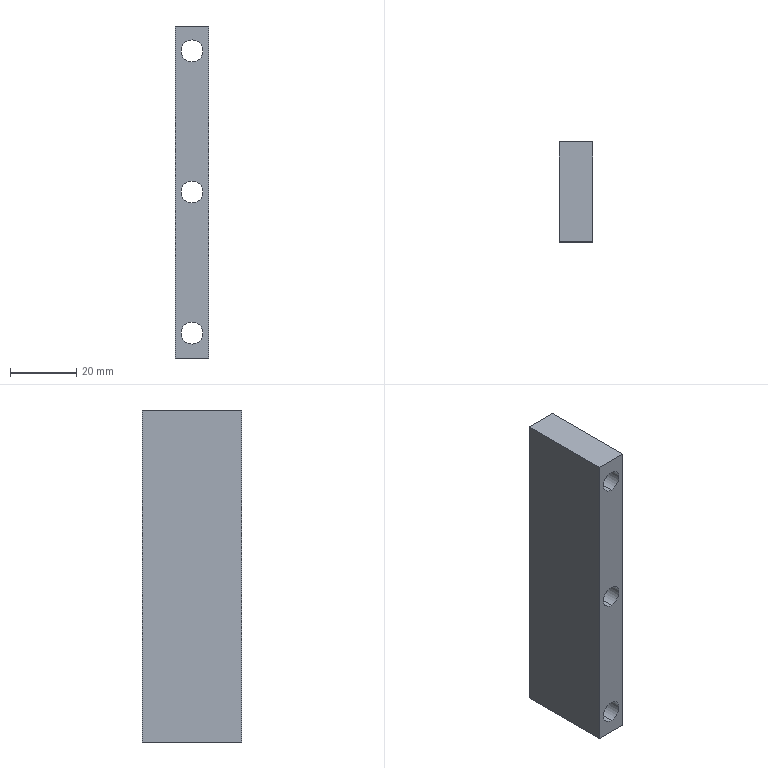Part | STEP file | 0-09-15 Support plate | 1 solid | 12 faces | box 10 x 30 x 100 mm | volume 26921 mm3 | cylinder 6 | plane 6 | commonest cylinder face diameters 6.6 x6
STEP:
#1=CARTESIAN_POINT('',(0.,0.,0.));
#2=DIRECTION('',(0.,0.,1.));
#3=DIRECTION('',(1.,0.,0.));
#4=AXIS2_PLACEMENT_3D('',#1,#2,#3);
#5=CARTESIAN_POINT('',(0.,-15.,-39.2));
#6=VERTEX_POINT('',#5);
#7=CARTESIAN_POINT('',(0.,15.,-39.2));
#8=VERTEX_POINT('',#7);
#9=CARTESIAN_POINT('',(0.,15.,-39.2));
#10=DIRECTION('',(0.,1.,0.));
#11=VECTOR('',#10,1.);
#12=LINE('',#9,#11);
#13=CARTESIAN_POINT('',(0.,15.,-42.5));
#14=DIRECTION('',(0.,1.,0.));
#15=DIRECTION('',(0.,0.,1.));
#16=AXIS2_PLACEMENT_3D('',#13,#14,#15);
#17=CYLINDRICAL_SURFACE('',#16,3.3);
#18=CARTESIAN_POINT('',(6.283,0.));
#19=DIRECTION('',(0.,1.));
#20=VECTOR('',#19,1.);
#21=LINE('',#18,#20);
#22=(GEOMETRIC_REPRESENTATION_CONTEXT(2)PARAMETRIC_REPRESENTATION_CONTEXT()REPRESENTATION_CONTEXT('',''));
#23=DEFINITIONAL_REPRESENTATION('',(#21),#22);
#24=PCURVE('',#17,#23);
#25=CARTESIAN_POINT('',(0.,15.,-42.5));
#26=DIRECTION('',(0.,1.,0.));
#27=DIRECTION('',(0.,0.,1.));
#28=AXIS2_PLACEMENT_3D('',#25,#26,#27);
#29=CYLINDRICAL_SURFACE('',#28,3.3);
#30=CARTESIAN_POINT('',(0.,0.));
#31=DIRECTION('',(0.,1.));
#32=VECTOR('',#31,1.);
#33=LINE('',#30,#32);
#34=(GEOMETRIC_REPRESENTATION_CONTEXT(2)PARAMETRIC_REPRESENTATION_CONTEXT()REPRESENTATION_CONTEXT('',''));
#35=DEFINITIONAL_REPRESENTATION('',(#33),#34);
#36=PCURVE('',#29,#35);
#37=SURFACE_CURVE('',#12,(#24,#36),.PCURVE_S1.);
#38=EDGE_CURVE('',#6,#8,#37,.T.);
#39=ORIENTED_EDGE('',*,*,#38,.T.);
#40=CARTESIAN_POINT('',(0.,15.,-45.8));
#41=VERTEX_POINT('',#40);
#42=CARTESIAN_POINT('',(0.,15.,-42.5));
#43=DIRECTION('',(0.,1.,0.));
#44=DIRECTION('',(0.,0.,1.));
#45=AXIS2_PLACEMENT_3D('',#42,#43,#44);
#46=CIRCLE('',#45,3.3);
#47=CARTESIAN_POINT('',(0.,0.));
#48=DIRECTION('',(1.,0.));
#49=VECTOR('',#48,1.);
#50=LINE('',#47,#49);
#51=(GEOMETRIC_REPRESENTATION_CONTEXT(2)PARAMETRIC_REPRESENTATION_CONTEXT()REPRESENTATION_CONTEXT('',''));
#52=DEFINITIONAL_REPRESENTATION('',(#50),#51);
#53=PCURVE('',#17,#52);
#54=CARTESIAN_POINT('',(5.,15.,-50.));
#55=DIRECTION('',(0.,-1.,0.));
#56=DIRECTION('',(0.,0.,-1.));
#57=AXIS2_PLACEMENT_3D('',#54,#55,#56);
#58=PLANE('',#57);
#59=CARTESIAN_POINT('',(-10.8,-5.));
#60=CARTESIAN_POINT('',(-10.8,0.7158));
#61=CARTESIAN_POINT('',(-5.85,-2.142));
#62=CARTESIAN_POINT('',(-0.9,-5.));
#63=CARTESIAN_POINT('',(-5.85,-7.858));
#64=CARTESIAN_POINT('',(-10.8,-10.716));
#65=CARTESIAN_POINT('',(-10.8,-5.));
#66=(BOUNDED_CURVE()B_SPLINE_CURVE(2,(#59,#60,#61,#62,#63,#64,#65),.UNSPECIFIED.,.T.,.F.)B_SPLINE_CURVE_WITH_KNOTS((1,2,2,2,2,1),(-2.094,0.,2.094,4.189,6.283,8.378),.UNSPECIFIED.)CURVE()GEOMETRIC_REPRESENTATION_ITEM()RATIONAL_B_SPLINE_CURVE((1.,0.5,1.,0.5,1.,0.5,1.))REPRESENTATION_ITEM(''));
#67=(GEOMETRIC_REPRESENTATION_CONTEXT(2)PARAMETRIC_REPRESENTATION_CONTEXT()REPRESENTATION_CONTEXT('',''));
#68=DEFINITIONAL_REPRESENTATION('',(#66),#67);
#69=PCURVE('',#58,#68);
#70=SURFACE_CURVE('',#46,(#53,#69),.PCURVE_S1.);
#71=EDGE_CURVE('',#41,#8,#70,.T.);
#72=ORIENTED_EDGE('',*,*,#71,.F.);
#73=CARTESIAN_POINT('',(0.,-15.,-45.8));
#74=VERTEX_POINT('',#73);
#75=CARTESIAN_POINT('',(0.,15.,-45.8));
#76=DIRECTION('',(0.,1.,0.));
#77=VECTOR('',#76,1.);
#78=LINE('',#75,#77);
#79=CARTESIAN_POINT('',(3.142,0.));
#80=DIRECTION('',(0.,1.));
#81=VECTOR('',#80,1.);
#82=LINE('',#79,#81);
#83=(GEOMETRIC_REPRESENTATION_CONTEXT(2)PARAMETRIC_REPRESENTATION_CONTEXT()REPRESENTATION_CONTEXT('',''));
#84=DEFINITIONAL_REPRESENTATION('',(#82),#83);
#85=PCURVE('',#17,#84);
#86=CARTESIAN_POINT('',(3.142,0.));
#87=DIRECTION('',(0.,1.));
#88=VECTOR('',#87,1.);
#89=LINE('',#86,#88);
#90=(GEOMETRIC_REPRESENTATION_CONTEXT(2)PARAMETRIC_REPRESENTATION_CONTEXT()REPRESENTATION_CONTEXT('',''));
#91=DEFINITIONAL_REPRESENTATION('',(#89),#90);
#92=PCURVE('',#29,#91);
#93=SURFACE_CURVE('',#78,(#85,#92),.PCURVE_S1.);
#94=EDGE_CURVE('',#74,#41,#93,.T.);
#95=ORIENTED_EDGE('',*,*,#94,.F.);
#96=CARTESIAN_POINT('',(0.,-15.,-42.5));
#97=DIRECTION('',(0.,1.,0.));
#98=DIRECTION('',(0.,0.,1.));
#99=AXIS2_PLACEMENT_3D('',#96,#97,#98);
#100=CIRCLE('',#99,3.3);
#101=CARTESIAN_POINT('',(0.,-30.));
#102=DIRECTION('',(1.,0.));
#103=VECTOR('',#102,1.);
#104=LINE('',#101,#103);
#105=(GEOMETRIC_REPRESENTATION_CONTEXT(2)PARAMETRIC_REPRESENTATION_CONTEXT()REPRESENTATION_CONTEXT('',''));
#106=DEFINITIONAL_REPRESENTATION('',(#104),#105);
#107=PCURVE('',#17,#106);
#108=CARTESIAN_POINT('',(5.,-15.,-50.));
#109=DIRECTION('',(0.,1.,0.));
#110=DIRECTION('',(0.,0.,1.));
#111=AXIS2_PLACEMENT_3D('',#108,#109,#110);
#112=PLANE('',#111);
#113=CARTESIAN_POINT('',(7.5,-5.));
#114=DIRECTION('',(1.,0.));
#115=AXIS2_PLACEMENT_2D('',#113,#114);
#116=CIRCLE('',#115,3.3);
#117=(GEOMETRIC_REPRESENTATION_CONTEXT(2)PARAMETRIC_REPRESENTATION_CONTEXT()REPRESENTATION_CONTEXT('',''));
#118=DEFINITIONAL_REPRESENTATION('',(#116),#117);
#119=PCURVE('',#112,#118);
#120=SURFACE_CURVE('',#100,(#107,#119),.PCURVE_S1.);
#121=EDGE_CURVE('',#74,#6,#120,.T.);
#122=ORIENTED_EDGE('',*,*,#121,.T.);
#123=EDGE_LOOP('',(#39,#72,#95,#122));
#124=FACE_BOUND('',#123,.F.);
#125=ADVANCED_FACE('',(#124),#17,.F.);
#126=CARTESIAN_POINT('',(0.,-15.,3.3));
#127=VERTEX_POINT('',#126);
#128=CARTESIAN_POINT('',(0.,15.,3.3));
#129=VERTEX_POINT('',#128);
#130=CARTESIAN_POINT('',(0.,15.,3.3));
#131=DIRECTION('',(0.,1.,0.));
#132=VECTOR('',#131,1.);
#133=LINE('',#130,#132);
#134=CARTESIAN_POINT('',(0.,15.,0.));
#135=DIRECTION('',(0.,1.,0.));
#136=DIRECTION('',(0.,0.,1.));
#137=AXIS2_PLACEMENT_3D('',#134,#135,#136);
#138=CYLINDRICAL_SURFACE('',#137,3.3);
#139=CARTESIAN_POINT('',(6.283,0.));
#140=DIRECTION('',(0.,1.));
#141=VECTOR('',#140,1.);
#142=LINE('',#139,#141);
#143=(GEOMETRIC_REPRESENTATION_CONTEXT(2)PARAMETRIC_REPRESENTATION_CONTEXT()REPRESENTATION_CONTEXT('',''));
#144=DEFINITIONAL_REPRESENTATION('',(#142),#143);
#145=PCURVE('',#138,#144);
#146=CARTESIAN_POINT('',(0.,15.,0.));
#147=DIRECTION('',(0.,1.,0.));
#148=DIRECTION('',(0.,0.,1.));
#149=AXIS2_PLACEMENT_3D('',#146,#147,#148);
#150=CYLINDRICAL_SURFACE('',#149,3.3);
#151=CARTESIAN_POINT('',(0.,0.));
#152=DIRECTION('',(0.,1.));
#153=VECTOR('',#152,1.);
#154=LINE('',#151,#153);
#155=(GEOMETRIC_REPRESENTATION_CONTEXT(2)PARAMETRIC_REPRESENTATION_CONTEXT()REPRESENTATION_CONTEXT('',''));
#156=DEFINITIONAL_REPRESENTATION('',(#154),#155);
#157=PCURVE('',#150,#156);
#158=SURFACE_CURVE('',#133,(#145,#157),.PCURVE_S1.);
#159=EDGE_CURVE('',#127,#129,#158,.T.);
#160=ORIENTED_EDGE('',*,*,#159,.T.);
#161=CARTESIAN_POINT('',(0.,15.,-3.3));
#162=VERTEX_POINT('',#161);
#163=CARTESIAN_POINT('',(0.,15.,0.));
#164=DIRECTION('',(0.,1.,0.));
#165=DIRECTION('',(0.,0.,1.));
#166=AXIS2_PLACEMENT_3D('',#163,#164,#165);
#167=CIRCLE('',#166,3.3);
#168=CARTESIAN_POINT('',(0.,0.));
#169=DIRECTION('',(1.,0.));
#170=VECTOR('',#169,1.);
#171=LINE('',#168,#170);
#172=(GEOMETRIC_REPRESENTATION_CONTEXT(2)PARAMETRIC_REPRESENTATION_CONTEXT()REPRESENTATION_CONTEXT('',''));
#173=DEFINITIONAL_REPRESENTATION('',(#171),#172);
#174=PCURVE('',#138,#173);
#175=CARTESIAN_POINT('',(-53.3,-5.));
#176=CARTESIAN_POINT('',(-53.3,0.7158));
#177=CARTESIAN_POINT('',(-48.35,-2.142));
#178=CARTESIAN_POINT('',(-43.4,-5.));
#179=CARTESIAN_POINT('',(-48.35,-7.858));
#180=CARTESIAN_POINT('',(-53.3,-10.716));
#181=CARTESIAN_POINT('',(-53.3,-5.));
#182=(BOUNDED_CURVE()B_SPLINE_CURVE(2,(#175,#176,#177,#178,#179,#180,#181),.UNSPECIFIED.,.T.,.F.)B_SPLINE_CURVE_WITH_KNOTS((1,2,2,2,2,1),(-2.094,0.,2.094,4.189,6.283,8.378),.UNSPECIFIED.)CURVE()GEOMETRIC_REPRESENTATION_ITEM()RATIONAL_B_SPLINE_CURVE((1.,0.5,1.,0.5,1.,0.5,1.))REPRESENTATION_ITEM(''));
#183=(GEOMETRIC_REPRESENTATION_CONTEXT(2)PARAMETRIC_REPRESENTATION_CONTEXT()REPRESENTATION_CONTEXT('',''));
#184=DEFINITIONAL_REPRESENTATION('',(#182),#183);
#185=PCURVE('',#58,#184);
#186=SURFACE_CURVE('',#167,(#174,#185),.PCURVE_S1.);
#187=EDGE_CURVE('',#162,#129,#186,.T.);
#188=ORIENTED_EDGE('',*,*,#187,.F.);
#189=CARTESIAN_POINT('',(0.,-15.,-3.3));
#190=VERTEX_POINT('',#189);
#191=CARTESIAN_POINT('',(0.,15.,-3.3));
#192=DIRECTION('',(0.,1.,0.));
#193=VECTOR('',#192,1.);
#194=LINE('',#191,#193);
#195=CARTESIAN_POINT('',(3.142,0.));
#196=DIRECTION('',(0.,1.));
#197=VECTOR('',#196,1.);
#198=LINE('',#195,#197);
#199=(GEOMETRIC_REPRESENTATION_CONTEXT(2)PARAMETRIC_REPRESENTATION_CONTEXT()REPRESENTATION_CONTEXT('',''));
#200=DEFINITIONAL_REPRESENTATION('',(#198),#199);
#201=PCURVE('',#138,#200);
#202=CARTESIAN_POINT('',(3.142,0.));
#203=DIRECTION('',(0.,1.));
#204=VECTOR('',#203,1.);
#205=LINE('',#202,#204);
#206=(GEOMETRIC_REPRESENTATION_CONTEXT(2)PARAMETRIC_REPRESENTATION_CONTEXT()REPRESENTATION_CONTEXT('',''));
#207=DEFINITIONAL_REPRESENTATION('',(#205),#206);
#208=PCURVE('',#150,#207);
#209=SURFACE_CURVE('',#194,(#201,#208),.PCURVE_S1.);
#210=EDGE_CURVE('',#190,#162,#209,.T.);
#211=ORIENTED_EDGE('',*,*,#210,.F.);
#212=CARTESIAN_POINT('',(0.,-15.,0.));
#213=DIRECTION('',(0.,1.,0.));
#214=DIRECTION('',(0.,0.,1.));
#215=AXIS2_PLACEMENT_3D('',#212,#213,#214);
#216=CIRCLE('',#215,3.3);
#217=CARTESIAN_POINT('',(0.,-30.));
#218=DIRECTION('',(1.,0.));
#219=VECTOR('',#218,1.);
#220=LINE('',#217,#219);
#221=(GEOMETRIC_REPRESENTATION_CONTEXT(2)PARAMETRIC_REPRESENTATION_CONTEXT()REPRESENTATION_CONTEXT('',''));
#222=DEFINITIONAL_REPRESENTATION('',(#220),#221);
#223=PCURVE('',#138,#222);
#224=CARTESIAN_POINT('',(50.,-5.));
#225=DIRECTION('',(1.,0.));
#226=AXIS2_PLACEMENT_2D('',#224,#225);
#227=CIRCLE('',#226,3.3);
#228=(GEOMETRIC_REPRESENTATION_CONTEXT(2)PARAMETRIC_REPRESENTATION_CONTEXT()REPRESENTATION_CONTEXT('',''));
#229=DEFINITIONAL_REPRESENTATION('',(#227),#228);
#230=PCURVE('',#112,#229);
#231=SURFACE_CURVE('',#216,(#223,#230),.PCURVE_S1.);
#232=EDGE_CURVE('',#190,#127,#231,.T.);
#233=ORIENTED_EDGE('',*,*,#232,.T.);
#234=EDGE_LOOP('',(#160,#188,#211,#233));
#235=FACE_BOUND('',#234,.F.);
#236=ADVANCED_FACE('',(#235),#138,.F.);
#237=CARTESIAN_POINT('',(0.,-15.,45.8));
#238=VERTEX_POINT('',#237);
#239=CARTESIAN_POINT('',(0.,15.,45.8));
#240=VERTEX_POINT('',#239);
#241=CARTESIAN_POINT('',(0.,15.,45.8));
#242=DIRECTION('',(0.,1.,0.));
#243=VECTOR('',#242,1.);
#244=LINE('',#241,#243);
#245=CARTESIAN_POINT('',(0.,15.,42.5));
#246=DIRECTION('',(0.,1.,0.));
#247=DIRECTION('',(0.,0.,1.));
#248=AXIS2_PLACEMENT_3D('',#245,#246,#247);
#249=CYLINDRICAL_SURFACE('',#248,3.3);
#250=CARTESIAN_POINT('',(6.283,0.));
#251=DIRECTION('',(0.,1.));
#252=VECTOR('',#251,1.);
#253=LINE('',#250,#252);
#254=(GEOMETRIC_REPRESENTATION_CONTEXT(2)PARAMETRIC_REPRESENTATION_CONTEXT()REPRESENTATION_CONTEXT('',''));
#255=DEFINITIONAL_REPRESENTATION('',(#253),#254);
#256=PCURVE('',#249,#255);
#257=CARTESIAN_POINT('',(0.,15.,42.5));
#258=DIRECTION('',(0.,1.,0.));
#259=DIRECTION('',(0.,0.,1.));
#260=AXIS2_PLACEMENT_3D('',#257,#258,#259);
#261=CYLINDRICAL_SURFACE('',#260,3.3);
#262=CARTESIAN_POINT('',(0.,0.));
#263=DIRECTION('',(0.,1.));
#264=VECTOR('',#263,1.);
#265=LINE('',#262,#264);
#266=(GEOMETRIC_REPRESENTATION_CONTEXT(2)PARAMETRIC_REPRESENTATION_CONTEXT()REPRESENTATION_CONTEXT('',''));
#267=DEFINITIONAL_REPRESENTATION('',(#265),#266);
#268=PCURVE('',#261,#267);
#269=SURFACE_CURVE('',#244,(#256,#268),.PCURVE_S1.);
#270=EDGE_CURVE('',#238,#240,#269,.T.);
#271=ORIENTED_EDGE('',*,*,#270,.T.);
#272=CARTESIAN_POINT('',(0.,15.,39.2));
#273=VERTEX_POINT('',#272);
#274=CARTESIAN_POINT('',(0.,15.,42.5));
#275=DIRECTION('',(0.,1.,0.));
#276=DIRECTION('',(0.,0.,1.));
#277=AXIS2_PLACEMENT_3D('',#274,#275,#276);
#278=CIRCLE('',#277,3.3);
#279=CARTESIAN_POINT('',(0.,0.));
#280=DIRECTION('',(1.,0.));
#281=VECTOR('',#280,1.);
#282=LINE('',#279,#281);
#283=(GEOMETRIC_REPRESENTATION_CONTEXT(2)PARAMETRIC_REPRESENTATION_CONTEXT()REPRESENTATION_CONTEXT('',''));
#284=DEFINITIONAL_REPRESENTATION('',(#282),#283);
#285=PCURVE('',#249,#284);
#286=CARTESIAN_POINT('',(-95.8,-5.));
#287=CARTESIAN_POINT('',(-95.8,0.7158));
#288=CARTESIAN_POINT('',(-90.85,-2.142));
#289=CARTESIAN_POINT('',(-85.9,-5.));
#290=CARTESIAN_POINT('',(-90.85,-7.858));
#291=CARTESIAN_POINT('',(-95.8,-10.716));
#292=CARTESIAN_POINT('',(-95.8,-5.));
#293=(BOUNDED_CURVE()B_SPLINE_CURVE(2,(#286,#287,#288,#289,#290,#291,#292),.UNSPECIFIED.,.T.,.F.)B_SPLINE_CURVE_WITH_KNOTS((1,2,2,2,2,1),(-2.094,0.,2.094,4.189,6.283,8.378),.UNSPECIFIED.)CURVE()GEOMETRIC_REPRESENTATION_ITEM()RATIONAL_B_SPLINE_CURVE((1.,0.5,1.,0.5,1.,0.5,1.))REPRESENTATION_ITEM(''));
#294=(GEOMETRIC_REPRESENTATION_CONTEXT(2)PARAMETRIC_REPRESENTATION_CONTEXT()REPRESENTATION_CONTEXT('',''));
#295=DEFINITIONAL_REPRESENTATION('',(#293),#294);
#296=PCURVE('',#58,#295);
#297=SURFACE_CURVE('',#278,(#285,#296),.PCURVE_S1.);
#298=EDGE_CURVE('',#273,#240,#297,.T.);
#299=ORIENTED_EDGE('',*,*,#298,.F.);
#300=CARTESIAN_POINT('',(0.,-15.,39.2));
#301=VERTEX_POINT('',#300);
#302=CARTESIAN_POINT('',(0.,15.,39.2));
#303=DIRECTION('',(0.,1.,0.));
#304=VECTOR('',#303,1.);
#305=LINE('',#302,#304);
#306=CARTESIAN_POINT('',(3.142,0.));
#307=DIRECTION('',(0.,1.));
#308=VECTOR('',#307,1.);
#309=LINE('',#306,#308);
#310=(GEOMETRIC_REPRESENTATION_CONTEXT(2)PARAMETRIC_REPRESENTATION_CONTEXT()REPRESENTATION_CONTEXT('',''));
#311=DEFINITIONAL_REPRESENTATION('',(#309),#310);
#312=PCURVE('',#249,#311);
#313=CARTESIAN_POINT('',(3.142,0.));
#314=DIRECTION('',(0.,1.));
#315=VECTOR('',#314,1.);
#316=LINE('',#313,#315);
#317=(GEOMETRIC_REPRESENTATION_CONTEXT(2)PARAMETRIC_REPRESENTATION_CONTEXT()REPRESENTATION_CONTEXT('',''));
#318=DEFINITIONAL_REPRESENTATION('',(#316),#317);
#319=PCURVE('',#261,#318);
#320=SURFACE_CURVE('',#305,(#312,#319),.PCURVE_S1.);
#321=EDGE_CURVE('',#301,#273,#320,.T.);
#322=ORIENTED_EDGE('',*,*,#321,.F.);
#323=CARTESIAN_POINT('',(0.,-15.,42.5));
#324=DIRECTION('',(0.,1.,0.));
#325=DIRECTION('',(0.,0.,1.));
#326=AXIS2_PLACEMENT_3D('',#323,#324,#325);
#327=CIRCLE('',#326,3.3);
#328=CARTESIAN_POINT('',(0.,-30.));
#329=DIRECTION('',(1.,0.));
#330=VECTOR('',#329,1.);
#331=LINE('',#328,#330);
#332=(GEOMETRIC_REPRESENTATION_CONTEXT(2)PARAMETRIC_REPRESENTATION_CONTEXT()REPRESENTATION_CONTEXT('',''));
#333=DEFINITIONAL_REPRESENTATION('',(#331),#332);
#334=PCURVE('',#249,#333);
#335=CARTESIAN_POINT('',(92.5,-5.));
#336=DIRECTION('',(1.,0.));
#337=AXIS2_PLACEMENT_2D('',#335,#336);
#338=CIRCLE('',#337,3.3);
#339=(GEOMETRIC_REPRESENTATION_CONTEXT(2)PARAMETRIC_REPRESENTATION_CONTEXT()REPRESENTATION_CONTEXT('',''));
#340=DEFINITIONAL_REPRESENTATION('',(#338),#339);
#341=PCURVE('',#112,#340);
#342=SURFACE_CURVE('',#327,(#334,#341),.PCURVE_S1.);
#343=EDGE_CURVE('',#301,#238,#342,.T.);
#344=ORIENTED_EDGE('',*,*,#343,.T.);
#345=EDGE_LOOP('',(#271,#299,#322,#344));
#346=FACE_BOUND('',#345,.F.);
#347=ADVANCED_FACE('',(#346),#249,.F.);
#348=CARTESIAN_POINT('',(-5.,15.,50.));
#349=VERTEX_POINT('',#348);
#350=CARTESIAN_POINT('',(-5.,-15.,50.));
#351=VERTEX_POINT('',#350);
#352=CARTESIAN_POINT('',(-5.,-15.,50.));
#353=DIRECTION('',(0.,-1.,0.));
#354=VECTOR('',#353,1.);
#355=LINE('',#352,#354);
#356=CARTESIAN_POINT('',(5.,-15.,50.));
#357=DIRECTION('',(0.,0.,-1.));
#358=DIRECTION('',(-1.,0.,0.));
#359=AXIS2_PLACEMENT_3D('',#356,#357,#358);
#360=PLANE('',#359);
#361=CARTESIAN_POINT('',(10.,0.));
#362=DIRECTION('',(0.,-1.));
#363=VECTOR('',#362,1.);
#364=LINE('',#361,#363);
#365=(GEOMETRIC_REPRESENTATION_CONTEXT(2)PARAMETRIC_REPRESENTATION_CONTEXT()REPRESENTATION_CONTEXT('',''));
#366=DEFINITIONAL_REPRESENTATION('',(#364),#365);
#367=PCURVE('',#360,#366);
#368=CARTESIAN_POINT('',(-5.,0.,0.));
#369=DIRECTION('',(1.,0.,0.));
#370=DIRECTION('',(0.,0.,-1.));
#371=AXIS2_PLACEMENT_3D('',#368,#369,#370);
#372=PLANE('',#371);
#373=CARTESIAN_POINT('',(-50.,-15.));
#374=DIRECTION('',(0.,-1.));
#375=VECTOR('',#374,1.);
#376=LINE('',#373,#375);
#377=(GEOMETRIC_REPRESENTATION_CONTEXT(2)PARAMETRIC_REPRESENTATION_CONTEXT()REPRESENTATION_CONTEXT('',''));
#378=DEFINITIONAL_REPRESENTATION('',(#376),#377);
#379=PCURVE('',#372,#378);
#380=SURFACE_CURVE('',#355,(#367,#379),.PCURVE_S1.);
#381=EDGE_CURVE('',#349,#351,#380,.T.);
#382=ORIENTED_EDGE('',*,*,#381,.T.);
#383=CARTESIAN_POINT('',(5.,-15.,50.));
#384=VERTEX_POINT('',#383);
#385=CARTESIAN_POINT('',(5.,-15.,50.));
#386=DIRECTION('',(-1.,0.,0.));
#387=VECTOR('',#386,1.);
#388=LINE('',#385,#387);
#389=CARTESIAN_POINT('',(0.,0.));
#390=DIRECTION('',(1.,0.));
#391=VECTOR('',#390,1.);
#392=LINE('',#389,#391);
#393=(GEOMETRIC_REPRESENTATION_CONTEXT(2)PARAMETRIC_REPRESENTATION_CONTEXT()REPRESENTATION_CONTEXT('',''));
#394=DEFINITIONAL_REPRESENTATION('',(#392),#393);
#395=PCURVE('',#360,#394);
#396=CARTESIAN_POINT('',(100.,0.));
#397=DIRECTION('',(0.,-1.));
#398=VECTOR('',#397,1.);
#399=LINE('',#396,#398);
#400=(GEOMETRIC_REPRESENTATION_CONTEXT(2)PARAMETRIC_REPRESENTATION_CONTEXT()REPRESENTATION_CONTEXT('',''));
#401=DEFINITIONAL_REPRESENTATION('',(#399),#400);
#402=PCURVE('',#112,#401);
#403=SURFACE_CURVE('',#388,(#395,#402),.PCURVE_S1.);
#404=EDGE_CURVE('',#384,#351,#403,.T.);
#405=ORIENTED_EDGE('',*,*,#404,.F.);
#406=CARTESIAN_POINT('',(5.,15.,50.));
#407=VERTEX_POINT('',#406);
#408=CARTESIAN_POINT('',(5.,-15.,50.));
#409=DIRECTION('',(0.,-1.,0.));
#410=VECTOR('',#409,1.);
#411=LINE('',#408,#410);
#412=CARTESIAN_POINT('',(0.,0.));
#413=DIRECTION('',(0.,-1.));
#414=VECTOR('',#413,1.);
#415=LINE('',#412,#414);
#416=(GEOMETRIC_REPRESENTATION_CONTEXT(2)PARAMETRIC_REPRESENTATION_CONTEXT()REPRESENTATION_CONTEXT('',''));
#417=DEFINITIONAL_REPRESENTATION('',(#415),#416);
#418=PCURVE('',#360,#417);
#419=CARTESIAN_POINT('',(5.,0.,0.));
#420=DIRECTION('',(1.,0.,0.));
#421=DIRECTION('',(0.,0.,-1.));
#422=AXIS2_PLACEMENT_3D('',#419,#420,#421);
#423=PLANE('',#422);
#424=CARTESIAN_POINT('',(-50.,-15.));
#425=DIRECTION('',(0.,-1.));
#426=VECTOR('',#425,1.);
#427=LINE('',#424,#426);
#428=(GEOMETRIC_REPRESENTATION_CONTEXT(2)PARAMETRIC_REPRESENTATION_CONTEXT()REPRESENTATION_CONTEXT('',''));
#429=DEFINITIONAL_REPRESENTATION('',(#427),#428);
#430=PCURVE('',#423,#429);
#431=SURFACE_CURVE('',#411,(#418,#430),.PCURVE_S1.);
#432=EDGE_CURVE('',#407,#384,#431,.T.);
#433=ORIENTED_EDGE('',*,*,#432,.F.);
#434=CARTESIAN_POINT('',(5.,15.,50.));
#435=DIRECTION('',(-1.,0.,0.));
#436=VECTOR('',#435,1.);
#437=LINE('',#434,#436);
#438=CARTESIAN_POINT('',(0.,30.));
#439=DIRECTION('',(1.,0.));
#440=VECTOR('',#439,1.);
#441=LINE('',#438,#440);
#442=(GEOMETRIC_REPRESENTATION_CONTEXT(2)PARAMETRIC_REPRESENTATION_CONTEXT()REPRESENTATION_CONTEXT('',''));
#443=DEFINITIONAL_REPRESENTATION('',(#441),#442);
#444=PCURVE('',#360,#443);
#445=CARTESIAN_POINT('',(-100.,0.));
#446=DIRECTION('',(0.,-1.));
#447=VECTOR('',#446,1.);
#448=LINE('',#445,#447);
#449=(GEOMETRIC_REPRESENTATION_CONTEXT(2)PARAMETRIC_REPRESENTATION_CONTEXT()REPRESENTATION_CONTEXT('',''));
#450=DEFINITIONAL_REPRESENTATION('',(#448),#449);
#451=PCURVE('',#58,#450);
#452=SURFACE_CURVE('',#437,(#444,#451),.PCURVE_S1.);
#453=EDGE_CURVE('',#407,#349,#452,.T.);
#454=ORIENTED_EDGE('',*,*,#453,.T.);
#455=EDGE_LOOP('',(#382,#405,#433,#454));
#456=FACE_BOUND('',#455,.T.);
#457=ADVANCED_FACE('',(#456),#360,.F.);
#458=CARTESIAN_POINT('',(0.,-15.,-42.5));
#459=DIRECTION('',(0.,1.,0.));
#460=DIRECTION('',(0.,0.,1.));
#461=AXIS2_PLACEMENT_3D('',#458,#459,#460);
#462=CIRCLE('',#461,3.3);
#463=CARTESIAN_POINT('',(7.5,-5.));
#464=DIRECTION('',(1.,0.));
#465=AXIS2_PLACEMENT_2D('',#463,#464);
#466=CIRCLE('',#465,3.3);
#467=(GEOMETRIC_REPRESENTATION_CONTEXT(2)PARAMETRIC_REPRESENTATION_CONTEXT()REPRESENTATION_CONTEXT('',''));
#468=DEFINITIONAL_REPRESENTATION('',(#466),#467);
#469=PCURVE('',#112,#468);
#470=CARTESIAN_POINT('',(0.,-30.));
#471=DIRECTION('',(1.,0.));
#472=VECTOR('',#471,1.);
#473=LINE('',#470,#472);
#474=(GEOMETRIC_REPRESENTATION_CONTEXT(2)PARAMETRIC_REPRESENTATION_CONTEXT()REPRESENTATION_CONTEXT('',''));
#475=DEFINITIONAL_REPRESENTATION('',(#473),#474);
#476=PCURVE('',#29,#475);
#477=SURFACE_CURVE('',#462,(#469,#476),.PCURVE_S1.);
#478=EDGE_CURVE('',#6,#74,#477,.T.);
#479=ORIENTED_EDGE('',*,*,#478,.T.);
#480=ORIENTED_EDGE('',*,*,#121,.T.);
#481=EDGE_LOOP('',(#479,#480));
#482=FACE_BOUND('',#481,.T.);
#483=CARTESIAN_POINT('',(0.,-15.,0.));
#484=DIRECTION('',(0.,1.,0.));
#485=DIRECTION('',(0.,0.,1.));
#486=AXIS2_PLACEMENT_3D('',#483,#484,#485);
#487=CIRCLE('',#486,3.3);
#488=CARTESIAN_POINT('',(50.,-5.));
#489=DIRECTION('',(1.,0.));
#490=AXIS2_PLACEMENT_2D('',#488,#489);
#491=CIRCLE('',#490,3.3);
#492=(GEOMETRIC_REPRESENTATION_CONTEXT(2)PARAMETRIC_REPRESENTATION_CONTEXT()REPRESENTATION_CONTEXT('',''));
#493=DEFINITIONAL_REPRESENTATION('',(#491),#492);
#494=PCURVE('',#112,#493);
#495=CARTESIAN_POINT('',(0.,-30.));
#496=DIRECTION('',(1.,0.));
#497=VECTOR('',#496,1.);
#498=LINE('',#495,#497);
#499=(GEOMETRIC_REPRESENTATION_CONTEXT(2)PARAMETRIC_REPRESENTATION_CONTEXT()REPRESENTATION_CONTEXT('',''));
#500=DEFINITIONAL_REPRESENTATION('',(#498),#499);
#501=PCURVE('',#150,#500);
#502=SURFACE_CURVE('',#487,(#494,#501),.PCURVE_S1.);
#503=EDGE_CURVE('',#127,#190,#502,.T.);
#504=ORIENTED_EDGE('',*,*,#503,.T.);
#505=ORIENTED_EDGE('',*,*,#232,.T.);
#506=EDGE_LOOP('',(#504,#505));
#507=FACE_BOUND('',#506,.T.);
#508=CARTESIAN_POINT('',(0.,-15.,42.5));
#509=DIRECTION('',(0.,1.,0.));
#510=DIRECTION('',(0.,0.,1.));
#511=AXIS2_PLACEMENT_3D('',#508,#509,#510);
#512=CIRCLE('',#511,3.3);
#513=CARTESIAN_POINT('',(92.5,-5.));
#514=DIRECTION('',(1.,0.));
#515=AXIS2_PLACEMENT_2D('',#513,#514);
#516=CIRCLE('',#515,3.3);
#517=(GEOMETRIC_REPRESENTATION_CONTEXT(2)PARAMETRIC_REPRESENTATION_CONTEXT()REPRESENTATION_CONTEXT('',''));
#518=DEFINITIONAL_REPRESENTATION('',(#516),#517);
#519=PCURVE('',#112,#518);
#520=CARTESIAN_POINT('',(0.,-30.));
#521=DIRECTION('',(1.,0.));
#522=VECTOR('',#521,1.);
#523=LINE('',#520,#522);
#524=(GEOMETRIC_REPRESENTATION_CONTEXT(2)PARAMETRIC_REPRESENTATION_CONTEXT()REPRESENTATION_CONTEXT('',''));
#525=DEFINITIONAL_REPRESENTATION('',(#523),#524);
#526=PCURVE('',#261,#525);
#527=SURFACE_CURVE('',#512,(#519,#526),.PCURVE_S1.);
#528=EDGE_CURVE('',#238,#301,#527,.T.);
#529=ORIENTED_EDGE('',*,*,#528,.T.);
#530=ORIENTED_EDGE('',*,*,#343,.T.);
#531=EDGE_LOOP('',(#529,#530));
#532=FACE_BOUND('',#531,.T.);
#533=CARTESIAN_POINT('',(-5.,-15.,-50.));
#534=VERTEX_POINT('',#533);
#535=CARTESIAN_POINT('',(-5.,-15.,-50.));
#536=DIRECTION('',(0.,0.,-1.));
#537=VECTOR('',#536,1.);
#538=LINE('',#535,#537);
#539=CARTESIAN_POINT('',(0.,-10.));
#540=DIRECTION('',(-1.,0.));
#541=VECTOR('',#540,1.);
#542=LINE('',#539,#541);
#543=(GEOMETRIC_REPRESENTATION_CONTEXT(2)PARAMETRIC_REPRESENTATION_CONTEXT()REPRESENTATION_CONTEXT('',''));
#544=DEFINITIONAL_REPRESENTATION('',(#542),#543);
#545=PCURVE('',#112,#544);
#546=CARTESIAN_POINT('',(50.,-15.));
#547=DIRECTION('',(1.,0.));
#548=VECTOR('',#547,1.);
#549=LINE('',#546,#548);
#550=(GEOMETRIC_REPRESENTATION_CONTEXT(2)PARAMETRIC_REPRESENTATION_CONTEXT()REPRESENTATION_CONTEXT('',''));
#551=DEFINITIONAL_REPRESENTATION('',(#549),#550);
#552=PCURVE('',#372,#551);
#553=SURFACE_CURVE('',#538,(#545,#552),.PCURVE_S1.);
#554=EDGE_CURVE('',#351,#534,#553,.T.);
#555=ORIENTED_EDGE('',*,*,#554,.T.);
#556=CARTESIAN_POINT('',(5.,-15.,-50.));
#557=VERTEX_POINT('',#556);
#558=CARTESIAN_POINT('',(5.,-15.,-50.));
#559=DIRECTION('',(-1.,0.,0.));
#560=VECTOR('',#559,1.);
#561=LINE('',#558,#560);
#562=CARTESIAN_POINT('',(0.,0.));
#563=DIRECTION('',(0.,-1.));
#564=VECTOR('',#563,1.);
#565=LINE('',#562,#564);
#566=(GEOMETRIC_REPRESENTATION_CONTEXT(2)PARAMETRIC_REPRESENTATION_CONTEXT()REPRESENTATION_CONTEXT('',''));
#567=DEFINITIONAL_REPRESENTATION('',(#565),#566);
#568=PCURVE('',#112,#567);
#569=CARTESIAN_POINT('',(5.,-15.,-50.));
#570=DIRECTION('',(0.,0.,1.));
#571=DIRECTION('',(1.,0.,0.));
#572=AXIS2_PLACEMENT_3D('',#569,#570,#571);
#573=PLANE('',#572);
#574=CARTESIAN_POINT('',(0.,0.));
#575=DIRECTION('',(-1.,0.));
#576=VECTOR('',#575,1.);
#577=LINE('',#574,#576);
#578=(GEOMETRIC_REPRESENTATION_CONTEXT(2)PARAMETRIC_REPRESENTATION_CONTEXT()REPRESENTATION_CONTEXT('',''));
#579=DEFINITIONAL_REPRESENTATION('',(#577),#578);
#580=PCURVE('',#573,#579);
#581=SURFACE_CURVE('',#561,(#568,#580),.PCURVE_S1.);
#582=EDGE_CURVE('',#557,#534,#581,.T.);
#583=ORIENTED_EDGE('',*,*,#582,.F.);
#584=CARTESIAN_POINT('',(5.,-15.,-50.));
#585=DIRECTION('',(0.,0.,-1.));
#586=VECTOR('',#585,1.);
#587=LINE('',#584,#586);
#588=CARTESIAN_POINT('',(0.,0.));
#589=DIRECTION('',(-1.,0.));
#590=VECTOR('',#589,1.);
#591=LINE('',#588,#590);
#592=(GEOMETRIC_REPRESENTATION_CONTEXT(2)PARAMETRIC_REPRESENTATION_CONTEXT()REPRESENTATION_CONTEXT('',''));
#593=DEFINITIONAL_REPRESENTATION('',(#591),#592);
#594=PCURVE('',#112,#593);
#595=CARTESIAN_POINT('',(50.,-15.));
#596=DIRECTION('',(1.,0.));
#597=VECTOR('',#596,1.);
#598=LINE('',#595,#597);
#599=(GEOMETRIC_REPRESENTATION_CONTEXT(2)PARAMETRIC_REPRESENTATION_CONTEXT()REPRESENTATION_CONTEXT('',''));
#600=DEFINITIONAL_REPRESENTATION('',(#598),#599);
#601=PCURVE('',#423,#600);
#602=SURFACE_CURVE('',#587,(#594,#601),.PCURVE_S1.);
#603=EDGE_CURVE('',#384,#557,#602,.T.);
#604=ORIENTED_EDGE('',*,*,#603,.F.);
#605=ORIENTED_EDGE('',*,*,#404,.T.);
#606=EDGE_LOOP('',(#555,#583,#604,#605));
#607=FACE_BOUND('',#606,.T.);
#608=ADVANCED_FACE('',(#482,#507,#532,#607),#112,.F.);
#609=CARTESIAN_POINT('',(-5.,15.,-50.));
#610=VERTEX_POINT('',#609);
#611=CARTESIAN_POINT('',(-5.,-15.,-50.));
#612=DIRECTION('',(0.,1.,0.));
#613=VECTOR('',#612,1.);
#614=LINE('',#611,#613);
#615=CARTESIAN_POINT('',(-10.,0.));
#616=DIRECTION('',(0.,1.));
#617=VECTOR('',#616,1.);
#618=LINE('',#615,#617);
#619=(GEOMETRIC_REPRESENTATION_CONTEXT(2)PARAMETRIC_REPRESENTATION_CONTEXT()REPRESENTATION_CONTEXT('',''));
#620=DEFINITIONAL_REPRESENTATION('',(#618),#619);
#621=PCURVE('',#573,#620);
#622=CARTESIAN_POINT('',(50.,-15.));
#623=DIRECTION('',(0.,1.));
#624=VECTOR('',#623,1.);
#625=LINE('',#622,#624);
#626=(GEOMETRIC_REPRESENTATION_CONTEXT(2)PARAMETRIC_REPRESENTATION_CONTEXT()REPRESENTATION_CONTEXT('',''));
#627=DEFINITIONAL_REPRESENTATION('',(#625),#626);
#628=PCURVE('',#372,#627);
#629=SURFACE_CURVE('',#614,(#621,#628),.PCURVE_S1.);
#630=EDGE_CURVE('',#534,#610,#629,.T.);
#631=ORIENTED_EDGE('',*,*,#630,.T.);
#632=CARTESIAN_POINT('',(5.,15.,-50.));
#633=VERTEX_POINT('',#632);
#634=CARTESIAN_POINT('',(5.,15.,-50.));
#635=DIRECTION('',(-1.,0.,0.));
#636=VECTOR('',#635,1.);
#637=LINE('',#634,#636);
#638=CARTESIAN_POINT('',(0.,30.));
#639=DIRECTION('',(-1.,0.));
#640=VECTOR('',#639,1.);
#641=LINE('',#638,#640);
#642=(GEOMETRIC_REPRESENTATION_CONTEXT(2)PARAMETRIC_REPRESENTATION_CONTEXT()REPRESENTATION_CONTEXT('',''));
#643=DEFINITIONAL_REPRESENTATION('',(#641),#642);
#644=PCURVE('',#573,#643);
#645=CARTESIAN_POINT('',(0.,0.));
#646=DIRECTION('',(0.,-1.));
#647=VECTOR('',#646,1.);
#648=LINE('',#645,#647);
#649=(GEOMETRIC_REPRESENTATION_CONTEXT(2)PARAMETRIC_REPRESENTATION_CONTEXT()REPRESENTATION_CONTEXT('',''));
#650=DEFINITIONAL_REPRESENTATION('',(#648),#649);
#651=PCURVE('',#58,#650);
#652=SURFACE_CURVE('',#637,(#644,#651),.PCURVE_S1.);
#653=EDGE_CURVE('',#633,#610,#652,.T.);
#654=ORIENTED_EDGE('',*,*,#653,.F.);
#655=CARTESIAN_POINT('',(5.,-15.,-50.));
#656=DIRECTION('',(0.,1.,0.));
#657=VECTOR('',#656,1.);
#658=LINE('',#655,#657);
#659=CARTESIAN_POINT('',(0.,0.));
#660=DIRECTION('',(0.,1.));
#661=VECTOR('',#660,1.);
#662=LINE('',#659,#661);
#663=(GEOMETRIC_REPRESENTATION_CONTEXT(2)PARAMETRIC_REPRESENTATION_CONTEXT()REPRESENTATION_CONTEXT('',''));
#664=DEFINITIONAL_REPRESENTATION('',(#662),#663);
#665=PCURVE('',#573,#664);
#666=CARTESIAN_POINT('',(50.,-15.));
#667=DIRECTION('',(0.,1.));
#668=VECTOR('',#667,1.);
#669=LINE('',#666,#668);
#670=(GEOMETRIC_REPRESENTATION_CONTEXT(2)PARAMETRIC_REPRESENTATION_CONTEXT()REPRESENTATION_CONTEXT('',''));
#671=DEFINITIONAL_REPRESENTATION('',(#669),#670);
#672=PCURVE('',#423,#671);
#673=SURFACE_CURVE('',#658,(#665,#672),.PCURVE_S1.);
#674=EDGE_CURVE('',#557,#633,#673,.T.);
#675=ORIENTED_EDGE('',*,*,#674,.F.);
#676=ORIENTED_EDGE('',*,*,#582,.T.);
#677=EDGE_LOOP('',(#631,#654,#675,#676));
#678=FACE_BOUND('',#677,.T.);
#679=ADVANCED_FACE('',(#678),#573,.F.);
#680=CARTESIAN_POINT('',(0.,15.,-42.5));
#681=DIRECTION('',(0.,1.,0.));
#682=DIRECTION('',(0.,0.,1.));
#683=AXIS2_PLACEMENT_3D('',#680,#681,#682);
#684=CIRCLE('',#683,3.3);
#685=CARTESIAN_POINT('',(-10.8,-5.));
#686=CARTESIAN_POINT('',(-10.8,0.7158));
#687=CARTESIAN_POINT('',(-5.85,-2.142));
#688=CARTESIAN_POINT('',(-0.9,-5.));
#689=CARTESIAN_POINT('',(-5.85,-7.858));
#690=CARTESIAN_POINT('',(-10.8,-10.716));
#691=CARTESIAN_POINT('',(-10.8,-5.));
#692=(BOUNDED_CURVE()B_SPLINE_CURVE(2,(#685,#686,#687,#688,#689,#690,#691),.UNSPECIFIED.,.T.,.F.)B_SPLINE_CURVE_WITH_KNOTS((1,2,2,2,2,1),(-2.094,0.,2.094,4.189,6.283,8.378),.UNSPECIFIED.)CURVE()GEOMETRIC_REPRESENTATION_ITEM()RATIONAL_B_SPLINE_CURVE((1.,0.5,1.,0.5,1.,0.5,1.))REPRESENTATION_ITEM(''));
#693=(GEOMETRIC_REPRESENTATION_CONTEXT(2)PARAMETRIC_REPRESENTATION_CONTEXT()REPRESENTATION_CONTEXT('',''));
#694=DEFINITIONAL_REPRESENTATION('',(#692),#693);
#695=PCURVE('',#58,#694);
#696=CARTESIAN_POINT('',(0.,0.));
#697=DIRECTION('',(1.,0.));
#698=VECTOR('',#697,1.);
#699=LINE('',#696,#698);
#700=(GEOMETRIC_REPRESENTATION_CONTEXT(2)PARAMETRIC_REPRESENTATION_CONTEXT()REPRESENTATION_CONTEXT('',''));
#701=DEFINITIONAL_REPRESENTATION('',(#699),#700);
#702=PCURVE('',#29,#701);
#703=SURFACE_CURVE('',#684,(#695,#702),.PCURVE_S1.);
#704=EDGE_CURVE('',#8,#41,#703,.T.);
#705=ORIENTED_EDGE('',*,*,#704,.F.);
#706=ORIENTED_EDGE('',*,*,#71,.F.);
#707=EDGE_LOOP('',(#705,#706));
#708=FACE_BOUND('',#707,.T.);
#709=CARTESIAN_POINT('',(0.,15.,0.));
#710=DIRECTION('',(0.,1.,0.));
#711=DIRECTION('',(0.,0.,1.));
#712=AXIS2_PLACEMENT_3D('',#709,#710,#711);
#713=CIRCLE('',#712,3.3);
#714=CARTESIAN_POINT('',(-53.3,-5.));
#715=CARTESIAN_POINT('',(-53.3,0.7158));
#716=CARTESIAN_POINT('',(-48.35,-2.142));
#717=CARTESIAN_POINT('',(-43.4,-5.));
#718=CARTESIAN_POINT('',(-48.35,-7.858));
#719=CARTESIAN_POINT('',(-53.3,-10.716));
#720=CARTESIAN_POINT('',(-53.3,-5.));
#721=(BOUNDED_CURVE()B_SPLINE_CURVE(2,(#714,#715,#716,#717,#718,#719,#720),.UNSPECIFIED.,.T.,.F.)B_SPLINE_CURVE_WITH_KNOTS((1,2,2,2,2,1),(-2.094,0.,2.094,4.189,6.283,8.378),.UNSPECIFIED.)CURVE()GEOMETRIC_REPRESENTATION_ITEM()RATIONAL_B_SPLINE_CURVE((1.,0.5,1.,0.5,1.,0.5,1.))REPRESENTATION_ITEM(''));
#722=(GEOMETRIC_REPRESENTATION_CONTEXT(2)PARAMETRIC_REPRESENTATION_CONTEXT()REPRESENTATION_CONTEXT('',''));
#723=DEFINITIONAL_REPRESENTATION('',(#721),#722);
#724=PCURVE('',#58,#723);
#725=CARTESIAN_POINT('',(0.,0.));
#726=DIRECTION('',(1.,0.));
#727=VECTOR('',#726,1.);
#728=LINE('',#725,#727);
#729=(GEOMETRIC_REPRESENTATION_CONTEXT(2)PARAMETRIC_REPRESENTATION_CONTEXT()REPRESENTATION_CONTEXT('',''));
#730=DEFINITIONAL_REPRESENTATION('',(#728),#729);
#731=PCURVE('',#150,#730);
#732=SURFACE_CURVE('',#713,(#724,#731),.PCURVE_S1.);
#733=EDGE_CURVE('',#129,#162,#732,.T.);
#734=ORIENTED_EDGE('',*,*,#733,.F.);
#735=ORIENTED_EDGE('',*,*,#187,.F.);
#736=EDGE_LOOP('',(#734,#735));
#737=FACE_BOUND('',#736,.T.);
#738=CARTESIAN_POINT('',(0.,15.,42.5));
#739=DIRECTION('',(0.,1.,0.));
#740=DIRECTION('',(0.,0.,1.));
#741=AXIS2_PLACEMENT_3D('',#738,#739,#740);
#742=CIRCLE('',#741,3.3);
#743=CARTESIAN_POINT('',(-95.8,-5.));
#744=CARTESIAN_POINT('',(-95.8,0.7158));
#745=CARTESIAN_POINT('',(-90.85,-2.142));
#746=CARTESIAN_POINT('',(-85.9,-5.));
#747=CARTESIAN_POINT('',(-90.85,-7.858));
#748=CARTESIAN_POINT('',(-95.8,-10.716));
#749=CARTESIAN_POINT('',(-95.8,-5.));
#750=(BOUNDED_CURVE()B_SPLINE_CURVE(2,(#743,#744,#745,#746,#747,#748,#749),.UNSPECIFIED.,.T.,.F.)B_SPLINE_CURVE_WITH_KNOTS((1,2,2,2,2,1),(-2.094,0.,2.094,4.189,6.283,8.378),.UNSPECIFIED.)CURVE()GEOMETRIC_REPRESENTATION_ITEM()RATIONAL_B_SPLINE_CURVE((1.,0.5,1.,0.5,1.,0.5,1.))REPRESENTATION_ITEM(''));
#751=(GEOMETRIC_REPRESENTATION_CONTEXT(2)PARAMETRIC_REPRESENTATION_CONTEXT()REPRESENTATION_CONTEXT('',''));
#752=DEFINITIONAL_REPRESENTATION('',(#750),#751);
#753=PCURVE('',#58,#752);
#754=CARTESIAN_POINT('',(0.,0.));
#755=DIRECTION('',(1.,0.));
#756=VECTOR('',#755,1.);
#757=LINE('',#754,#756);
#758=(GEOMETRIC_REPRESENTATION_CONTEXT(2)PARAMETRIC_REPRESENTATION_CONTEXT()REPRESENTATION_CONTEXT('',''));
#759=DEFINITIONAL_REPRESENTATION('',(#757),#758);
#760=PCURVE('',#261,#759);
#761=SURFACE_CURVE('',#742,(#753,#760),.PCURVE_S1.);
#762=EDGE_CURVE('',#240,#273,#761,.T.);
#763=ORIENTED_EDGE('',*,*,#762,.F.);
#764=ORIENTED_EDGE('',*,*,#298,.F.);
#765=EDGE_LOOP('',(#763,#764));
#766=FACE_BOUND('',#765,.T.);
#767=CARTESIAN_POINT('',(-5.,15.,-50.));
#768=DIRECTION('',(0.,0.,1.));
#769=VECTOR('',#768,1.);
#770=LINE('',#767,#769);
#771=CARTESIAN_POINT('',(0.,-10.));
#772=DIRECTION('',(-1.,0.));
#773=VECTOR('',#772,1.);
#774=LINE('',#771,#773);
#775=(GEOMETRIC_REPRESENTATION_CONTEXT(2)PARAMETRIC_REPRESENTATION_CONTEXT()REPRESENTATION_CONTEXT('',''));
#776=DEFINITIONAL_REPRESENTATION('',(#774),#775);
#777=PCURVE('',#58,#776);
#778=CARTESIAN_POINT('',(50.,15.));
#779=DIRECTION('',(-1.,0.));
#780=VECTOR('',#779,1.);
#781=LINE('',#778,#780);
#782=(GEOMETRIC_REPRESENTATION_CONTEXT(2)PARAMETRIC_REPRESENTATION_CONTEXT()REPRESENTATION_CONTEXT('',''));
#783=DEFINITIONAL_REPRESENTATION('',(#781),#782);
#784=PCURVE('',#372,#783);
#785=SURFACE_CURVE('',#770,(#777,#784),.PCURVE_S1.);
#786=EDGE_CURVE('',#610,#349,#785,.T.);
#787=ORIENTED_EDGE('',*,*,#786,.T.);
#788=ORIENTED_EDGE('',*,*,#453,.F.);
#789=CARTESIAN_POINT('',(5.,15.,-50.));
#790=DIRECTION('',(0.,0.,1.));
#791=VECTOR('',#790,1.);
#792=LINE('',#789,#791);
#793=CARTESIAN_POINT('',(0.,0.));
#794=DIRECTION('',(-1.,0.));
#795=VECTOR('',#794,1.);
#796=LINE('',#793,#795);
#797=(GEOMETRIC_REPRESENTATION_CONTEXT(2)PARAMETRIC_REPRESENTATION_CONTEXT()REPRESENTATION_CONTEXT('',''));
#798=DEFINITIONAL_REPRESENTATION('',(#796),#797);
#799=PCURVE('',#58,#798);
#800=CARTESIAN_POINT('',(50.,15.));
#801=DIRECTION('',(-1.,0.));
#802=VECTOR('',#801,1.);
#803=LINE('',#800,#802);
#804=(GEOMETRIC_REPRESENTATION_CONTEXT(2)PARAMETRIC_REPRESENTATION_CONTEXT()REPRESENTATION_CONTEXT('',''));
#805=DEFINITIONAL_REPRESENTATION('',(#803),#804);
#806=PCURVE('',#423,#805);
#807=SURFACE_CURVE('',#792,(#799,#806),.PCURVE_S1.);
#808=EDGE_CURVE('',#633,#407,#807,.T.);
#809=ORIENTED_EDGE('',*,*,#808,.F.);
#810=ORIENTED_EDGE('',*,*,#653,.T.);
#811=EDGE_LOOP('',(#787,#788,#809,#810));
#812=FACE_BOUND('',#811,.T.);
#813=ADVANCED_FACE('',(#708,#737,#766,#812),#58,.F.);
#814=ORIENTED_EDGE('',*,*,#432,.T.);
#815=ORIENTED_EDGE('',*,*,#603,.T.);
#816=ORIENTED_EDGE('',*,*,#674,.T.);
#817=ORIENTED_EDGE('',*,*,#808,.T.);
#818=EDGE_LOOP('',(#814,#815,#816,#817));
#819=FACE_BOUND('',#818,.T.);
#820=ADVANCED_FACE('',(#819),#423,.T.);
#821=ORIENTED_EDGE('',*,*,#381,.F.);
#822=ORIENTED_EDGE('',*,*,#786,.F.);
#823=ORIENTED_EDGE('',*,*,#630,.F.);
#824=ORIENTED_EDGE('',*,*,#554,.F.);
#825=EDGE_LOOP('',(#821,#822,#823,#824));
#826=FACE_BOUND('',#825,.T.);
#827=ADVANCED_FACE('',(#826),#372,.F.);
#828=ORIENTED_EDGE('',*,*,#762,.F.);
#829=ORIENTED_EDGE('',*,*,#270,.F.);
#830=ORIENTED_EDGE('',*,*,#528,.T.);
#831=ORIENTED_EDGE('',*,*,#321,.T.);
#832=EDGE_LOOP('',(#828,#829,#830,#831));
#833=FACE_BOUND('',#832,.F.);
#834=ADVANCED_FACE('',(#833),#261,.F.);
#835=ORIENTED_EDGE('',*,*,#733,.F.);
#836=ORIENTED_EDGE('',*,*,#159,.F.);
#837=ORIENTED_EDGE('',*,*,#503,.T.);
#838=ORIENTED_EDGE('',*,*,#210,.T.);
#839=EDGE_LOOP('',(#835,#836,#837,#838));
#840=FACE_BOUND('',#839,.F.);
#841=ADVANCED_FACE('',(#840),#150,.F.);
#842=ORIENTED_EDGE('',*,*,#704,.F.);
#843=ORIENTED_EDGE('',*,*,#38,.F.);
#844=ORIENTED_EDGE('',*,*,#478,.T.);
#845=ORIENTED_EDGE('',*,*,#94,.T.);
#846=EDGE_LOOP('',(#842,#843,#844,#845));
#847=FACE_BOUND('',#846,.F.);
#848=ADVANCED_FACE('',(#847),#29,.F.);
#849=CLOSED_SHELL('',(#125,#236,#347,#457,#608,#679,#813,#820,#827,#834,#841,#848));
#850=MANIFOLD_SOLID_BREP('',#849);
#851=(LENGTH_UNIT()NAMED_UNIT(*)SI_UNIT(.MILLI.,.METRE.));
#852=UNCERTAINTY_MEASURE_WITH_UNIT(LENGTH_MEASURE(0.0000001),#851,'','');
#853=(NAMED_UNIT(*)PLANE_ANGLE_UNIT()SI_UNIT($,.RADIAN.));
#854=(NAMED_UNIT(*)SI_UNIT($,.STERADIAN.)SOLID_ANGLE_UNIT());
#855=(GEOMETRIC_REPRESENTATION_CONTEXT(3)GLOBAL_UNCERTAINTY_ASSIGNED_CONTEXT((#852))GLOBAL_UNIT_ASSIGNED_CONTEXT((#851,#853,#854))REPRESENTATION_CONTEXT('',''));
#856=ADVANCED_BREP_SHAPE_REPRESENTATION('',(#4,#850),#855);